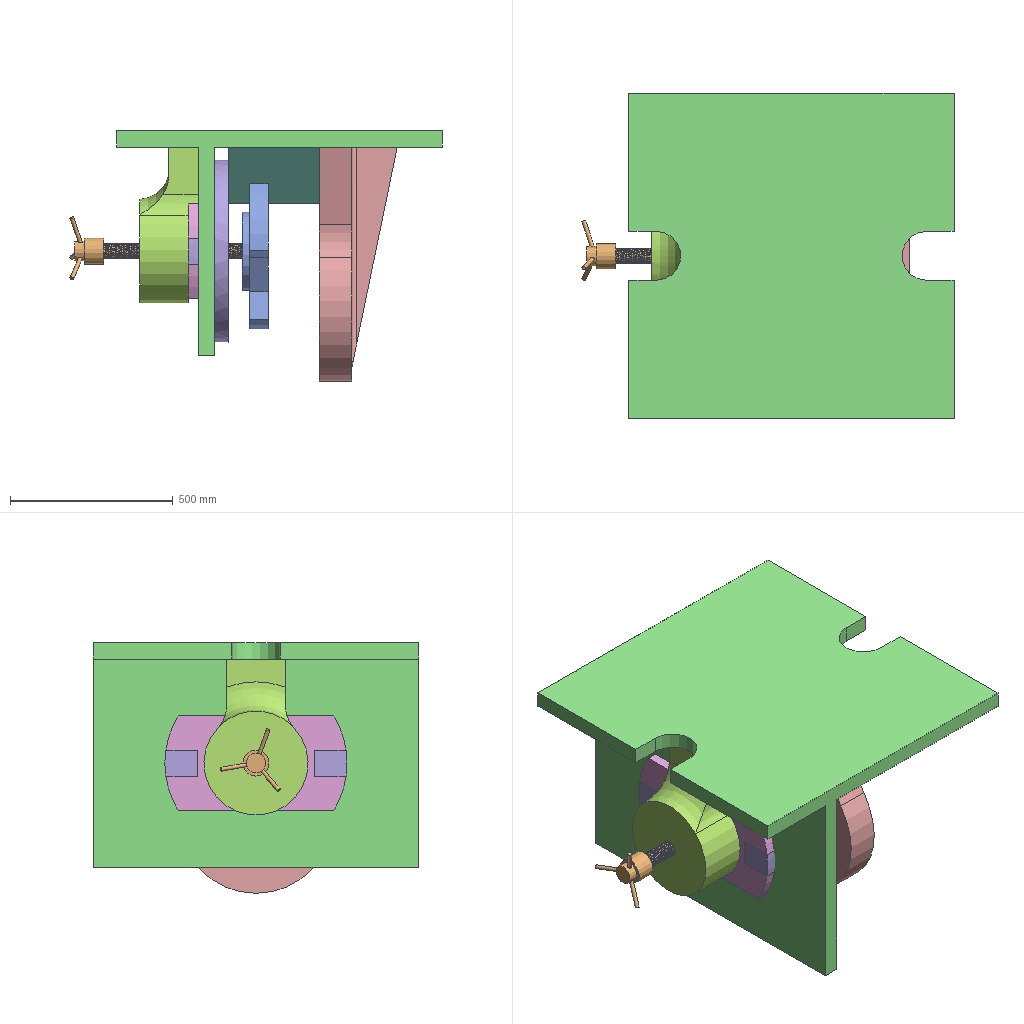Assembly | NX | 9 different items | 9 placed | box 1144 x 1000 x 770 mm
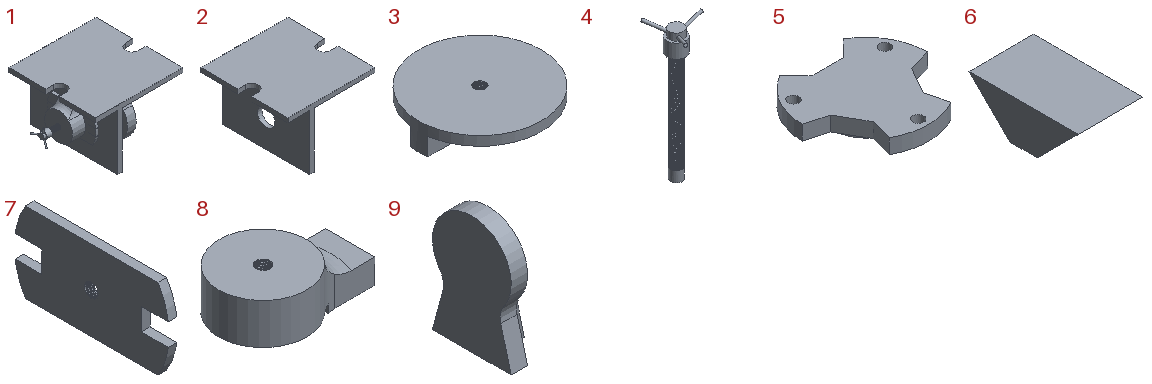Parts list (item | quantity | size | volume | features):
1 | x1 | 1144 x 1000 x 770 mm | 170686521 mm3 | features DATUM_CSYS 22, EXTRUDE 14, SKETCH 14, CYLINDER 12, DATUM_PLANE 8, BLEND 5, HELIX 4, SWP104 4, EXTRACT_BODY 2, Pattern Geometry 1, UNITE 1
2 | x1 | 1000 x 1000 x 690 mm | 78270631 mm3 | features DATUM_CSYS 4, EXTRUDE 3, SKETCH 3, DATUM_PLANE 2, BLEND 1
3 | x1 | 560 x 560 x 123 mm | 13014650 mm3 | features DATUM_CSYS 3, CYLINDER 2, EXTRUDE 2, SKETCH 2, HELIX 1, SWP104 1
4 | x1 | 170.632 x 195.599 x 574.025 mm | 1187331 mm3 | features CYLINDER 4, DATUM_CSYS 3, DATUM_PLANE 3, EXTRACT_BODY 2, SKETCH 2, EXTRUDE 1, HELIX 1, Pattern Geometry 1, SWP104 1, UNITE 1
5 | x1 | 479.982 x 446.798 x 80 mm | 8098473 mm3 | features CYLINDER 3, DATUM_CSYS 2, EXTRUDE 1, SKETCH 1
6 | x1 | 280 x 470 x 175 mm | 14455000 mm3 | features DATUM_CSYS 2, DATUM_PLANE 1, EXTRUDE 1, SKETCH 1
7 | x1 | 31 x 554.256 x 290 mm | 4245966 mm3 | features DATUM_CSYS 2, EXTRUDE 2, DATUM_PLANE 1, HELIX 1, SKETCH 1, SWP104 1
8 | x1 | 480 x 320 x 180 mm | 14833518 mm3 | features DATUM_CSYS 3, BLEND 2, CYLINDER 2, EXTRUDE 2, SKETCH 2, DATUM_PLANE 1, HELIX 1, SWP104 1
9 | x1 | 240 x 480 x 720 mm | 36580765 mm3 | features DATUM_CSYS 3, BLEND 2, EXTRUDE 2, SKETCH 2, CYLINDER 1
Mates (type | each side: item.copy, entity, surface, feature):
Touch | 3.1 face cylinder Cylinder(1) | 2.1 face cylinder Extrude(6)
Parallel | 3.1 face plane Extrude(4) | 2.1 face plane Extrude(2)
Touch | 3.1 face plane Cylinder(1) | 2.1 face plane Extrude(2)
Touch | 4.1 face cylinder Cylinder(1) | 3.1 face cylinder Cylinder(1)
Touch | 7.1 face plane Extrude(3) | 2.1 face plane Extrude(2)
Touch | 7.1 face cylinder Extrude(4) | 4.1 face cylinder Cylinder(1)
Parallel | 7.1 face plane Extrude(3) | 2.1 face plane Extrude(2)
Touch | 8.1 face cylinder Cylinder(1) | 4.1 face cylinder Cylinder(1)
Touch | 8.1 face plane Extrude(3) | 2.1 face plane Extrude(2)
Touch | 8.1 face plane Cylinder(1) | 2.1 face plane Extrude(2)
Parallel | 5.1 face plane Extrude(2) | 2.1 face plane Extrude(2)
Touch | 5.1 face cylinder Cylinder(5) | 4.1 face cylinder Cylinder(7)
Touch | 5.1 face plane Cylinder(5) | 4.1 face plane Cylinder(7)
Touch | 6.1 face plane Extrude(2) | 3.1 face plane Cylinder(1)
Distance | 4.1 face plane Cylinder(2) | 8.1 face plane Cylinder(1)
Touch | 9.1 face plane Extrude(1) | 2.1 face plane Extrude(2)
Touch | 9.1 face plane Extrude(1) | 6.1 face plane Extrude(2)
Center22 | 9.1 face plane Extrude(3) | 9.1 face plane Extrude(3) | 2.1 face plane Extrude(2) | 2.1 face plane Extrude(2)